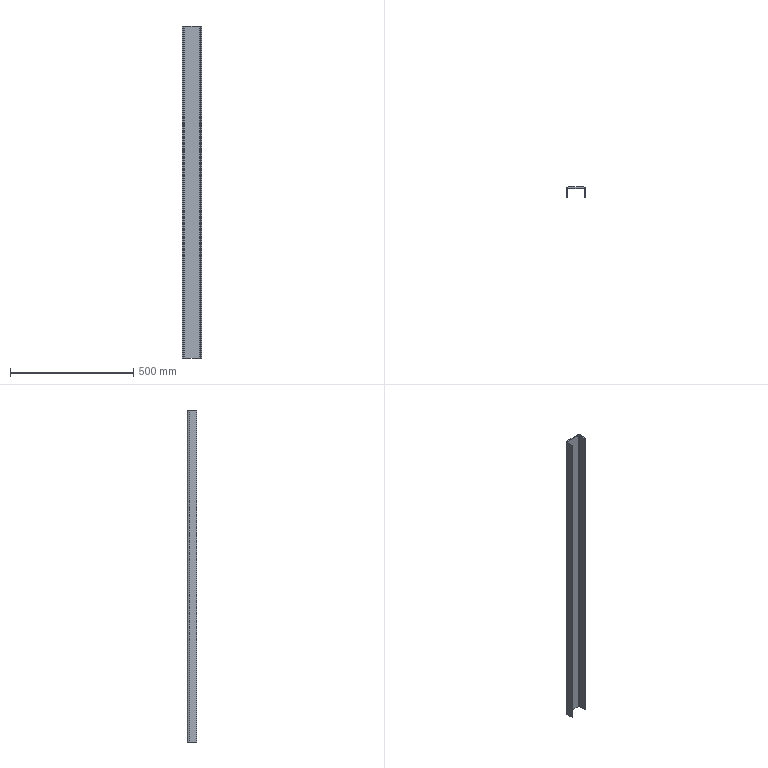Part | STEP file | 1 solid | 14 faces | box 80 x 40 x 1349 mm | volume 968325 mm3 | plane 10 | cylinder 4 | commonest cylinder face diameters 10 x2 20 x2
STEP:
#1=CARTESIAN_POINT('',(0.,0.,0.));
#2=DIRECTION('',(0.,0.,1.));
#3=DIRECTION('',(1.,0.,0.));
#4=AXIS2_PLACEMENT_3D('',#1,#2,#3);
#5=CARTESIAN_POINT('',(-35.,0.,674.5));
#6=VERTEX_POINT('',#5);
#7=CARTESIAN_POINT('',(-40.,0.,674.5));
#8=VERTEX_POINT('',#7);
#9=CARTESIAN_POINT('',(-30.,0.,674.5));
#10=DIRECTION('',(-1.,0.,0.));
#11=VECTOR('',#10,1.);
#12=LINE('',#9,#11);
#13=CARTESIAN_POINT('',(-35.,0.,674.5));
#14=DIRECTION('',(0.,-1.,0.));
#15=DIRECTION('',(0.,0.,-1.));
#16=AXIS2_PLACEMENT_3D('',#13,#14,#15);
#17=PLANE('',#16);
#18=CARTESIAN_POINT('',(0.,5.));
#19=DIRECTION('',(0.,-1.));
#20=VECTOR('',#19,1.);
#21=LINE('',#18,#20);
#22=(GEOMETRIC_REPRESENTATION_CONTEXT(2)PARAMETRIC_REPRESENTATION_CONTEXT()REPRESENTATION_CONTEXT('',''));
#23=DEFINITIONAL_REPRESENTATION('',(#21),#22);
#24=PCURVE('',#17,#23);
#25=CARTESIAN_POINT('',(-30.,30.,674.5));
#26=DIRECTION('',(0.,0.,-1.));
#27=DIRECTION('',(0.,-1.,0.));
#28=AXIS2_PLACEMENT_3D('',#25,#26,#27);
#29=PLANE('',#28);
#30=CARTESIAN_POINT('',(30.,0.));
#31=DIRECTION('',(0.,1.));
#32=VECTOR('',#31,1.);
#33=LINE('',#30,#32);
#34=(GEOMETRIC_REPRESENTATION_CONTEXT(2)PARAMETRIC_REPRESENTATION_CONTEXT()REPRESENTATION_CONTEXT('',''));
#35=DEFINITIONAL_REPRESENTATION('',(#33),#34);
#36=PCURVE('',#29,#35);
#37=SURFACE_CURVE('',#12,(#24,#36),.PCURVE_S1.);
#38=EDGE_CURVE('',#6,#8,#37,.T.);
#39=ORIENTED_EDGE('',*,*,#38,.T.);
#40=CARTESIAN_POINT('',(-40.,0.,-674.5));
#41=VERTEX_POINT('',#40);
#42=CARTESIAN_POINT('',(-40.,0.,674.5));
#43=DIRECTION('',(0.,0.,1.));
#44=VECTOR('',#43,1.);
#45=LINE('',#42,#44);
#46=CARTESIAN_POINT('',(0.,-5.));
#47=DIRECTION('',(-1.,0.));
#48=VECTOR('',#47,1.);
#49=LINE('',#46,#48);
#50=(GEOMETRIC_REPRESENTATION_CONTEXT(2)PARAMETRIC_REPRESENTATION_CONTEXT()REPRESENTATION_CONTEXT('',''));
#51=DEFINITIONAL_REPRESENTATION('',(#49),#50);
#52=PCURVE('',#17,#51);
#53=CARTESIAN_POINT('',(-40.,0.,674.5));
#54=DIRECTION('',(-1.,0.,0.));
#55=DIRECTION('',(0.,0.,1.));
#56=AXIS2_PLACEMENT_3D('',#53,#54,#55);
#57=PLANE('',#56);
#58=CARTESIAN_POINT('',(0.,0.));
#59=DIRECTION('',(1.,0.));
#60=VECTOR('',#59,1.);
#61=LINE('',#58,#60);
#62=(GEOMETRIC_REPRESENTATION_CONTEXT(2)PARAMETRIC_REPRESENTATION_CONTEXT()REPRESENTATION_CONTEXT('',''));
#63=DEFINITIONAL_REPRESENTATION('',(#61),#62);
#64=PCURVE('',#57,#63);
#65=SURFACE_CURVE('',#45,(#52,#64),.PCURVE_S1.);
#66=EDGE_CURVE('',#41,#8,#65,.T.);
#67=ORIENTED_EDGE('',*,*,#66,.F.);
#68=CARTESIAN_POINT('',(-35.,0.,-674.5));
#69=VERTEX_POINT('',#68);
#70=CARTESIAN_POINT('',(-30.,0.,-674.5));
#71=DIRECTION('',(-1.,0.,0.));
#72=VECTOR('',#71,1.);
#73=LINE('',#70,#72);
#74=CARTESIAN_POINT('',(1349.,5.));
#75=DIRECTION('',(0.,-1.));
#76=VECTOR('',#75,1.);
#77=LINE('',#74,#76);
#78=(GEOMETRIC_REPRESENTATION_CONTEXT(2)PARAMETRIC_REPRESENTATION_CONTEXT()REPRESENTATION_CONTEXT('',''));
#79=DEFINITIONAL_REPRESENTATION('',(#77),#78);
#80=PCURVE('',#17,#79);
#81=CARTESIAN_POINT('',(-30.,30.,-674.5));
#82=DIRECTION('',(0.,0.,-1.));
#83=DIRECTION('',(0.,-1.,0.));
#84=AXIS2_PLACEMENT_3D('',#81,#82,#83);
#85=PLANE('',#84);
#86=CARTESIAN_POINT('',(30.,0.));
#87=DIRECTION('',(0.,1.));
#88=VECTOR('',#87,1.);
#89=LINE('',#86,#88);
#90=(GEOMETRIC_REPRESENTATION_CONTEXT(2)PARAMETRIC_REPRESENTATION_CONTEXT()REPRESENTATION_CONTEXT('',''));
#91=DEFINITIONAL_REPRESENTATION('',(#89),#90);
#92=PCURVE('',#85,#91);
#93=SURFACE_CURVE('',#73,(#80,#92),.PCURVE_S1.);
#94=EDGE_CURVE('',#69,#41,#93,.T.);
#95=ORIENTED_EDGE('',*,*,#94,.F.);
#96=CARTESIAN_POINT('',(-35.,0.,674.5));
#97=DIRECTION('',(0.,0.,-1.));
#98=VECTOR('',#97,1.);
#99=LINE('',#96,#98);
#100=CARTESIAN_POINT('',(0.,0.));
#101=DIRECTION('',(1.,0.));
#102=VECTOR('',#101,1.);
#103=LINE('',#100,#102);
#104=(GEOMETRIC_REPRESENTATION_CONTEXT(2)PARAMETRIC_REPRESENTATION_CONTEXT()REPRESENTATION_CONTEXT('',''));
#105=DEFINITIONAL_REPRESENTATION('',(#103),#104);
#106=PCURVE('',#17,#105);
#107=CARTESIAN_POINT('',(-35.,30.,674.5));
#108=DIRECTION('',(1.,0.,0.));
#109=DIRECTION('',(0.,1.,0.));
#110=AXIS2_PLACEMENT_3D('',#107,#108,#109);
#111=PLANE('',#110);
#112=CARTESIAN_POINT('',(-30.,0.));
#113=DIRECTION('',(0.,-1.));
#114=VECTOR('',#113,1.);
#115=LINE('',#112,#114);
#116=(GEOMETRIC_REPRESENTATION_CONTEXT(2)PARAMETRIC_REPRESENTATION_CONTEXT()REPRESENTATION_CONTEXT('',''));
#117=DEFINITIONAL_REPRESENTATION('',(#115),#116);
#118=PCURVE('',#111,#117);
#119=SURFACE_CURVE('',#99,(#106,#118),.PCURVE_S1.);
#120=EDGE_CURVE('',#6,#69,#119,.T.);
#121=ORIENTED_EDGE('',*,*,#120,.F.);
#122=EDGE_LOOP('',(#39,#67,#95,#121));
#123=FACE_BOUND('',#122,.T.);
#124=ADVANCED_FACE('',(#123),#17,.T.);
#125=CARTESIAN_POINT('',(-40.,30.,674.5));
#126=VERTEX_POINT('',#125);
#127=CARTESIAN_POINT('',(-40.,30.,674.5));
#128=DIRECTION('',(0.,1.,0.));
#129=VECTOR('',#128,1.);
#130=LINE('',#127,#129);
#131=CARTESIAN_POINT('',(0.,30.));
#132=DIRECTION('',(0.,1.));
#133=VECTOR('',#132,1.);
#134=LINE('',#131,#133);
#135=(GEOMETRIC_REPRESENTATION_CONTEXT(2)PARAMETRIC_REPRESENTATION_CONTEXT()REPRESENTATION_CONTEXT('',''));
#136=DEFINITIONAL_REPRESENTATION('',(#134),#135);
#137=PCURVE('',#57,#136);
#138=CARTESIAN_POINT('',(0.,10.));
#139=DIRECTION('',(-1.,0.));
#140=VECTOR('',#139,1.);
#141=LINE('',#138,#140);
#142=(GEOMETRIC_REPRESENTATION_CONTEXT(2)PARAMETRIC_REPRESENTATION_CONTEXT()REPRESENTATION_CONTEXT('',''));
#143=DEFINITIONAL_REPRESENTATION('',(#141),#142);
#144=PCURVE('',#29,#143);
#145=SURFACE_CURVE('',#130,(#137,#144),.PCURVE_S1.);
#146=EDGE_CURVE('',#8,#126,#145,.T.);
#147=ORIENTED_EDGE('',*,*,#146,.T.);
#148=CARTESIAN_POINT('',(-40.,30.,-674.5));
#149=VERTEX_POINT('',#148);
#150=CARTESIAN_POINT('',(-40.,30.,674.5));
#151=DIRECTION('',(0.,0.,1.));
#152=VECTOR('',#151,1.);
#153=LINE('',#150,#152);
#154=CARTESIAN_POINT('',(0.,30.));
#155=DIRECTION('',(1.,0.));
#156=VECTOR('',#155,1.);
#157=LINE('',#154,#156);
#158=(GEOMETRIC_REPRESENTATION_CONTEXT(2)PARAMETRIC_REPRESENTATION_CONTEXT()REPRESENTATION_CONTEXT('',''));
#159=DEFINITIONAL_REPRESENTATION('',(#157),#158);
#160=PCURVE('',#57,#159);
#161=CARTESIAN_POINT('',(-30.,30.,674.5));
#162=DIRECTION('',(0.,0.,-1.));
#163=DIRECTION('',(-1.,0.,0.));
#164=AXIS2_PLACEMENT_3D('',#161,#162,#163);
#165=CYLINDRICAL_SURFACE('',#164,10.);
#166=CARTESIAN_POINT('',(0.,0.));
#167=DIRECTION('',(0.,-1.));
#168=VECTOR('',#167,1.);
#169=LINE('',#166,#168);
#170=(GEOMETRIC_REPRESENTATION_CONTEXT(2)PARAMETRIC_REPRESENTATION_CONTEXT()REPRESENTATION_CONTEXT('',''));
#171=DEFINITIONAL_REPRESENTATION('',(#169),#170);
#172=PCURVE('',#165,#171);
#173=SURFACE_CURVE('',#153,(#160,#172),.PCURVE_S1.);
#174=EDGE_CURVE('',#149,#126,#173,.T.);
#175=ORIENTED_EDGE('',*,*,#174,.F.);
#176=CARTESIAN_POINT('',(-40.,30.,-674.5));
#177=DIRECTION('',(0.,1.,0.));
#178=VECTOR('',#177,1.);
#179=LINE('',#176,#178);
#180=CARTESIAN_POINT('',(-1349.,30.));
#181=DIRECTION('',(0.,1.));
#182=VECTOR('',#181,1.);
#183=LINE('',#180,#182);
#184=(GEOMETRIC_REPRESENTATION_CONTEXT(2)PARAMETRIC_REPRESENTATION_CONTEXT()REPRESENTATION_CONTEXT('',''));
#185=DEFINITIONAL_REPRESENTATION('',(#183),#184);
#186=PCURVE('',#57,#185);
#187=CARTESIAN_POINT('',(0.,10.));
#188=DIRECTION('',(-1.,0.));
#189=VECTOR('',#188,1.);
#190=LINE('',#187,#189);
#191=(GEOMETRIC_REPRESENTATION_CONTEXT(2)PARAMETRIC_REPRESENTATION_CONTEXT()REPRESENTATION_CONTEXT('',''));
#192=DEFINITIONAL_REPRESENTATION('',(#190),#191);
#193=PCURVE('',#85,#192);
#194=SURFACE_CURVE('',#179,(#186,#193),.PCURVE_S1.);
#195=EDGE_CURVE('',#41,#149,#194,.T.);
#196=ORIENTED_EDGE('',*,*,#195,.F.);
#197=ORIENTED_EDGE('',*,*,#66,.T.);
#198=EDGE_LOOP('',(#147,#175,#196,#197));
#199=FACE_BOUND('',#198,.T.);
#200=ADVANCED_FACE('',(#199),#57,.T.);
#201=CARTESIAN_POINT('',(-30.,40.,674.5));
#202=VERTEX_POINT('',#201);
#203=CARTESIAN_POINT('',(-30.,30.,674.5));
#204=DIRECTION('',(0.,0.,-1.));
#205=DIRECTION('',(-1.,0.,0.));
#206=AXIS2_PLACEMENT_3D('',#203,#204,#205);
#207=CIRCLE('',#206,10.);
#208=CARTESIAN_POINT('',(0.,0.));
#209=DIRECTION('',(1.,0.));
#210=VECTOR('',#209,1.);
#211=LINE('',#208,#210);
#212=(GEOMETRIC_REPRESENTATION_CONTEXT(2)PARAMETRIC_REPRESENTATION_CONTEXT()REPRESENTATION_CONTEXT('',''));
#213=DEFINITIONAL_REPRESENTATION('',(#211),#212);
#214=PCURVE('',#165,#213);
#215=CARTESIAN_POINT('',(0.,0.));
#216=DIRECTION('',(0.,1.));
#217=AXIS2_PLACEMENT_2D('',#215,#216);
#218=CIRCLE('',#217,10.);
#219=(GEOMETRIC_REPRESENTATION_CONTEXT(2)PARAMETRIC_REPRESENTATION_CONTEXT()REPRESENTATION_CONTEXT('',''));
#220=DEFINITIONAL_REPRESENTATION('',(#218),#219);
#221=PCURVE('',#29,#220);
#222=SURFACE_CURVE('',#207,(#214,#221),.PCURVE_S1.);
#223=EDGE_CURVE('',#126,#202,#222,.T.);
#224=ORIENTED_EDGE('',*,*,#223,.T.);
#225=CARTESIAN_POINT('',(-30.,40.,-674.5));
#226=VERTEX_POINT('',#225);
#227=CARTESIAN_POINT('',(-30.,40.,674.5));
#228=DIRECTION('',(0.,0.,1.));
#229=VECTOR('',#228,1.);
#230=LINE('',#227,#229);
#231=CARTESIAN_POINT('',(1.571,0.));
#232=DIRECTION('',(0.,-1.));
#233=VECTOR('',#232,1.);
#234=LINE('',#231,#233);
#235=(GEOMETRIC_REPRESENTATION_CONTEXT(2)PARAMETRIC_REPRESENTATION_CONTEXT()REPRESENTATION_CONTEXT('',''));
#236=DEFINITIONAL_REPRESENTATION('',(#234),#235);
#237=PCURVE('',#165,#236);
#238=CARTESIAN_POINT('',(-30.,40.,674.5));
#239=DIRECTION('',(0.,1.,0.));
#240=DIRECTION('',(1.,0.,0.));
#241=AXIS2_PLACEMENT_3D('',#238,#239,#240);
#242=PLANE('',#241);
#243=CARTESIAN_POINT('',(0.,0.));
#244=DIRECTION('',(0.,-1.));
#245=VECTOR('',#244,1.);
#246=LINE('',#243,#245);
#247=(GEOMETRIC_REPRESENTATION_CONTEXT(2)PARAMETRIC_REPRESENTATION_CONTEXT()REPRESENTATION_CONTEXT('',''));
#248=DEFINITIONAL_REPRESENTATION('',(#246),#247);
#249=PCURVE('',#242,#248);
#250=SURFACE_CURVE('',#230,(#237,#249),.PCURVE_S1.);
#251=EDGE_CURVE('',#226,#202,#250,.T.);
#252=ORIENTED_EDGE('',*,*,#251,.F.);
#253=CARTESIAN_POINT('',(-30.,30.,-674.5));
#254=DIRECTION('',(0.,0.,-1.));
#255=DIRECTION('',(-1.,0.,0.));
#256=AXIS2_PLACEMENT_3D('',#253,#254,#255);
#257=CIRCLE('',#256,10.);
#258=CARTESIAN_POINT('',(0.,1349.));
#259=DIRECTION('',(1.,0.));
#260=VECTOR('',#259,1.);
#261=LINE('',#258,#260);
#262=(GEOMETRIC_REPRESENTATION_CONTEXT(2)PARAMETRIC_REPRESENTATION_CONTEXT()REPRESENTATION_CONTEXT('',''));
#263=DEFINITIONAL_REPRESENTATION('',(#261),#262);
#264=PCURVE('',#165,#263);
#265=CARTESIAN_POINT('',(0.,0.));
#266=DIRECTION('',(0.,1.));
#267=AXIS2_PLACEMENT_2D('',#265,#266);
#268=CIRCLE('',#267,10.);
#269=(GEOMETRIC_REPRESENTATION_CONTEXT(2)PARAMETRIC_REPRESENTATION_CONTEXT()REPRESENTATION_CONTEXT('',''));
#270=DEFINITIONAL_REPRESENTATION('',(#268),#269);
#271=PCURVE('',#85,#270);
#272=SURFACE_CURVE('',#257,(#264,#271),.PCURVE_S1.);
#273=EDGE_CURVE('',#149,#226,#272,.T.);
#274=ORIENTED_EDGE('',*,*,#273,.F.);
#275=ORIENTED_EDGE('',*,*,#174,.T.);
#276=EDGE_LOOP('',(#224,#252,#274,#275));
#277=FACE_BOUND('',#276,.T.);
#278=ADVANCED_FACE('',(#277),#165,.T.);
#279=CARTESIAN_POINT('',(30.,40.,674.5));
#280=VERTEX_POINT('',#279);
#281=CARTESIAN_POINT('',(-30.,40.,674.5));
#282=DIRECTION('',(1.,0.,0.));
#283=VECTOR('',#282,1.);
#284=LINE('',#281,#283);
#285=CARTESIAN_POINT('',(0.,0.));
#286=DIRECTION('',(1.,0.));
#287=VECTOR('',#286,1.);
#288=LINE('',#285,#287);
#289=(GEOMETRIC_REPRESENTATION_CONTEXT(2)PARAMETRIC_REPRESENTATION_CONTEXT()REPRESENTATION_CONTEXT('',''));
#290=DEFINITIONAL_REPRESENTATION('',(#288),#289);
#291=PCURVE('',#242,#290);
#292=CARTESIAN_POINT('',(-10.,0.));
#293=DIRECTION('',(0.,-1.));
#294=VECTOR('',#293,1.);
#295=LINE('',#292,#294);
#296=(GEOMETRIC_REPRESENTATION_CONTEXT(2)PARAMETRIC_REPRESENTATION_CONTEXT()REPRESENTATION_CONTEXT('',''));
#297=DEFINITIONAL_REPRESENTATION('',(#295),#296);
#298=PCURVE('',#29,#297);
#299=SURFACE_CURVE('',#284,(#291,#298),.PCURVE_S1.);
#300=EDGE_CURVE('',#202,#280,#299,.T.);
#301=ORIENTED_EDGE('',*,*,#300,.T.);
#302=CARTESIAN_POINT('',(30.,40.,-674.5));
#303=VERTEX_POINT('',#302);
#304=CARTESIAN_POINT('',(30.,40.,674.5));
#305=DIRECTION('',(0.,0.,1.));
#306=VECTOR('',#305,1.);
#307=LINE('',#304,#306);
#308=CARTESIAN_POINT('',(60.,0.));
#309=DIRECTION('',(0.,-1.));
#310=VECTOR('',#309,1.);
#311=LINE('',#308,#310);
#312=(GEOMETRIC_REPRESENTATION_CONTEXT(2)PARAMETRIC_REPRESENTATION_CONTEXT()REPRESENTATION_CONTEXT('',''));
#313=DEFINITIONAL_REPRESENTATION('',(#311),#312);
#314=PCURVE('',#242,#313);
#315=CARTESIAN_POINT('',(30.,30.,674.5));
#316=DIRECTION('',(0.,0.,-1.));
#317=DIRECTION('',(-1.,0.,0.));
#318=AXIS2_PLACEMENT_3D('',#315,#316,#317);
#319=CYLINDRICAL_SURFACE('',#318,10.);
#320=CARTESIAN_POINT('',(1.571,0.));
#321=DIRECTION('',(0.,-1.));
#322=VECTOR('',#321,1.);
#323=LINE('',#320,#322);
#324=(GEOMETRIC_REPRESENTATION_CONTEXT(2)PARAMETRIC_REPRESENTATION_CONTEXT()REPRESENTATION_CONTEXT('',''));
#325=DEFINITIONAL_REPRESENTATION('',(#323),#324);
#326=PCURVE('',#319,#325);
#327=SURFACE_CURVE('',#307,(#314,#326),.PCURVE_S1.);
#328=EDGE_CURVE('',#303,#280,#327,.T.);
#329=ORIENTED_EDGE('',*,*,#328,.F.);
#330=CARTESIAN_POINT('',(-30.,40.,-674.5));
#331=DIRECTION('',(1.,0.,0.));
#332=VECTOR('',#331,1.);
#333=LINE('',#330,#332);
#334=CARTESIAN_POINT('',(0.,1349.));
#335=DIRECTION('',(1.,0.));
#336=VECTOR('',#335,1.);
#337=LINE('',#334,#336);
#338=(GEOMETRIC_REPRESENTATION_CONTEXT(2)PARAMETRIC_REPRESENTATION_CONTEXT()REPRESENTATION_CONTEXT('',''));
#339=DEFINITIONAL_REPRESENTATION('',(#337),#338);
#340=PCURVE('',#242,#339);
#341=CARTESIAN_POINT('',(-10.,0.));
#342=DIRECTION('',(0.,-1.));
#343=VECTOR('',#342,1.);
#344=LINE('',#341,#343);
#345=(GEOMETRIC_REPRESENTATION_CONTEXT(2)PARAMETRIC_REPRESENTATION_CONTEXT()REPRESENTATION_CONTEXT('',''));
#346=DEFINITIONAL_REPRESENTATION('',(#344),#345);
#347=PCURVE('',#85,#346);
#348=SURFACE_CURVE('',#333,(#340,#347),.PCURVE_S1.);
#349=EDGE_CURVE('',#226,#303,#348,.T.);
#350=ORIENTED_EDGE('',*,*,#349,.F.);
#351=ORIENTED_EDGE('',*,*,#251,.T.);
#352=EDGE_LOOP('',(#301,#329,#350,#351));
#353=FACE_BOUND('',#352,.T.);
#354=ADVANCED_FACE('',(#353),#242,.T.);
#355=CARTESIAN_POINT('',(40.,30.,674.5));
#356=VERTEX_POINT('',#355);
#357=CARTESIAN_POINT('',(30.,30.,674.5));
#358=DIRECTION('',(0.,0.,-1.));
#359=DIRECTION('',(-1.,0.,0.));
#360=AXIS2_PLACEMENT_3D('',#357,#358,#359);
#361=CIRCLE('',#360,10.);
#362=CARTESIAN_POINT('',(0.,0.));
#363=DIRECTION('',(1.,0.));
#364=VECTOR('',#363,1.);
#365=LINE('',#362,#364);
#366=(GEOMETRIC_REPRESENTATION_CONTEXT(2)PARAMETRIC_REPRESENTATION_CONTEXT()REPRESENTATION_CONTEXT('',''));
#367=DEFINITIONAL_REPRESENTATION('',(#365),#366);
#368=PCURVE('',#319,#367);
#369=CARTESIAN_POINT('',(0.,-60.));
#370=DIRECTION('',(0.,1.));
#371=AXIS2_PLACEMENT_2D('',#369,#370);
#372=CIRCLE('',#371,10.);
#373=(GEOMETRIC_REPRESENTATION_CONTEXT(2)PARAMETRIC_REPRESENTATION_CONTEXT()REPRESENTATION_CONTEXT('',''));
#374=DEFINITIONAL_REPRESENTATION('',(#372),#373);
#375=PCURVE('',#29,#374);
#376=SURFACE_CURVE('',#361,(#368,#375),.PCURVE_S1.);
#377=EDGE_CURVE('',#280,#356,#376,.T.);
#378=ORIENTED_EDGE('',*,*,#377,.T.);
#379=CARTESIAN_POINT('',(40.,30.,-674.5));
#380=VERTEX_POINT('',#379);
#381=CARTESIAN_POINT('',(40.,30.,674.5));
#382=DIRECTION('',(0.,0.,1.));
#383=VECTOR('',#382,1.);
#384=LINE('',#381,#383);
#385=CARTESIAN_POINT('',(3.142,0.));
#386=DIRECTION('',(0.,-1.));
#387=VECTOR('',#386,1.);
#388=LINE('',#385,#387);
#389=(GEOMETRIC_REPRESENTATION_CONTEXT(2)PARAMETRIC_REPRESENTATION_CONTEXT()REPRESENTATION_CONTEXT('',''));
#390=DEFINITIONAL_REPRESENTATION('',(#388),#389);
#391=PCURVE('',#319,#390);
#392=CARTESIAN_POINT('',(40.,30.,674.5));
#393=DIRECTION('',(1.,0.,0.));
#394=DIRECTION('',(0.,-1.,0.));
#395=AXIS2_PLACEMENT_3D('',#392,#393,#394);
#396=PLANE('',#395);
#397=CARTESIAN_POINT('',(0.,0.));
#398=DIRECTION('',(0.,-1.));
#399=VECTOR('',#398,1.);
#400=LINE('',#397,#399);
#401=(GEOMETRIC_REPRESENTATION_CONTEXT(2)PARAMETRIC_REPRESENTATION_CONTEXT()REPRESENTATION_CONTEXT('',''));
#402=DEFINITIONAL_REPRESENTATION('',(#400),#401);
#403=PCURVE('',#396,#402);
#404=SURFACE_CURVE('',#384,(#391,#403),.PCURVE_S1.);
#405=EDGE_CURVE('',#380,#356,#404,.T.);
#406=ORIENTED_EDGE('',*,*,#405,.F.);
#407=CARTESIAN_POINT('',(30.,30.,-674.5));
#408=DIRECTION('',(0.,0.,-1.));
#409=DIRECTION('',(-1.,0.,0.));
#410=AXIS2_PLACEMENT_3D('',#407,#408,#409);
#411=CIRCLE('',#410,10.);
#412=CARTESIAN_POINT('',(0.,1349.));
#413=DIRECTION('',(1.,0.));
#414=VECTOR('',#413,1.);
#415=LINE('',#412,#414);
#416=(GEOMETRIC_REPRESENTATION_CONTEXT(2)PARAMETRIC_REPRESENTATION_CONTEXT()REPRESENTATION_CONTEXT('',''));
#417=DEFINITIONAL_REPRESENTATION('',(#415),#416);
#418=PCURVE('',#319,#417);
#419=CARTESIAN_POINT('',(0.,-60.));
#420=DIRECTION('',(0.,1.));
#421=AXIS2_PLACEMENT_2D('',#419,#420);
#422=CIRCLE('',#421,10.);
#423=(GEOMETRIC_REPRESENTATION_CONTEXT(2)PARAMETRIC_REPRESENTATION_CONTEXT()REPRESENTATION_CONTEXT('',''));
#424=DEFINITIONAL_REPRESENTATION('',(#422),#423);
#425=PCURVE('',#85,#424);
#426=SURFACE_CURVE('',#411,(#418,#425),.PCURVE_S1.);
#427=EDGE_CURVE('',#303,#380,#426,.T.);
#428=ORIENTED_EDGE('',*,*,#427,.F.);
#429=ORIENTED_EDGE('',*,*,#328,.T.);
#430=EDGE_LOOP('',(#378,#406,#428,#429));
#431=FACE_BOUND('',#430,.T.);
#432=ADVANCED_FACE('',(#431),#319,.T.);
#433=CARTESIAN_POINT('',(40.,0.,674.5));
#434=VERTEX_POINT('',#433);
#435=CARTESIAN_POINT('',(40.,30.,674.5));
#436=DIRECTION('',(0.,-1.,0.));
#437=VECTOR('',#436,1.);
#438=LINE('',#435,#437);
#439=CARTESIAN_POINT('',(0.,0.));
#440=DIRECTION('',(1.,0.));
#441=VECTOR('',#440,1.);
#442=LINE('',#439,#441);
#443=(GEOMETRIC_REPRESENTATION_CONTEXT(2)PARAMETRIC_REPRESENTATION_CONTEXT()REPRESENTATION_CONTEXT('',''));
#444=DEFINITIONAL_REPRESENTATION('',(#442),#443);
#445=PCURVE('',#396,#444);
#446=CARTESIAN_POINT('',(0.,-70.));
#447=DIRECTION('',(1.,0.));
#448=VECTOR('',#447,1.);
#449=LINE('',#446,#448);
#450=(GEOMETRIC_REPRESENTATION_CONTEXT(2)PARAMETRIC_REPRESENTATION_CONTEXT()REPRESENTATION_CONTEXT('',''));
#451=DEFINITIONAL_REPRESENTATION('',(#449),#450);
#452=PCURVE('',#29,#451);
#453=SURFACE_CURVE('',#438,(#445,#452),.PCURVE_S1.);
#454=EDGE_CURVE('',#356,#434,#453,.T.);
#455=ORIENTED_EDGE('',*,*,#454,.T.);
#456=CARTESIAN_POINT('',(40.,0.,-674.5));
#457=VERTEX_POINT('',#456);
#458=CARTESIAN_POINT('',(40.,0.,674.5));
#459=DIRECTION('',(0.,0.,1.));
#460=VECTOR('',#459,1.);
#461=LINE('',#458,#460);
#462=CARTESIAN_POINT('',(30.,0.));
#463=DIRECTION('',(0.,-1.));
#464=VECTOR('',#463,1.);
#465=LINE('',#462,#464);
#466=(GEOMETRIC_REPRESENTATION_CONTEXT(2)PARAMETRIC_REPRESENTATION_CONTEXT()REPRESENTATION_CONTEXT('',''));
#467=DEFINITIONAL_REPRESENTATION('',(#465),#466);
#468=PCURVE('',#396,#467);
#469=CARTESIAN_POINT('',(40.,0.,674.5));
#470=DIRECTION('',(0.,-1.,0.));
#471=DIRECTION('',(0.,0.,-1.));
#472=AXIS2_PLACEMENT_3D('',#469,#470,#471);
#473=PLANE('',#472);
#474=CARTESIAN_POINT('',(0.,0.));
#475=DIRECTION('',(-1.,0.));
#476=VECTOR('',#475,1.);
#477=LINE('',#474,#476);
#478=(GEOMETRIC_REPRESENTATION_CONTEXT(2)PARAMETRIC_REPRESENTATION_CONTEXT()REPRESENTATION_CONTEXT('',''));
#479=DEFINITIONAL_REPRESENTATION('',(#477),#478);
#480=PCURVE('',#473,#479);
#481=SURFACE_CURVE('',#461,(#468,#480),.PCURVE_S1.);
#482=EDGE_CURVE('',#457,#434,#481,.T.);
#483=ORIENTED_EDGE('',*,*,#482,.F.);
#484=CARTESIAN_POINT('',(40.,30.,-674.5));
#485=DIRECTION('',(0.,-1.,0.));
#486=VECTOR('',#485,1.);
#487=LINE('',#484,#486);
#488=CARTESIAN_POINT('',(0.,1349.));
#489=DIRECTION('',(1.,0.));
#490=VECTOR('',#489,1.);
#491=LINE('',#488,#490);
#492=(GEOMETRIC_REPRESENTATION_CONTEXT(2)PARAMETRIC_REPRESENTATION_CONTEXT()REPRESENTATION_CONTEXT('',''));
#493=DEFINITIONAL_REPRESENTATION('',(#491),#492);
#494=PCURVE('',#396,#493);
#495=CARTESIAN_POINT('',(0.,-70.));
#496=DIRECTION('',(1.,0.));
#497=VECTOR('',#496,1.);
#498=LINE('',#495,#497);
#499=(GEOMETRIC_REPRESENTATION_CONTEXT(2)PARAMETRIC_REPRESENTATION_CONTEXT()REPRESENTATION_CONTEXT('',''));
#500=DEFINITIONAL_REPRESENTATION('',(#498),#499);
#501=PCURVE('',#85,#500);
#502=SURFACE_CURVE('',#487,(#494,#501),.PCURVE_S1.);
#503=EDGE_CURVE('',#380,#457,#502,.T.);
#504=ORIENTED_EDGE('',*,*,#503,.F.);
#505=ORIENTED_EDGE('',*,*,#405,.T.);
#506=EDGE_LOOP('',(#455,#483,#504,#505));
#507=FACE_BOUND('',#506,.T.);
#508=ADVANCED_FACE('',(#507),#396,.T.);
#509=CARTESIAN_POINT('',(35.,0.,674.5));
#510=VERTEX_POINT('',#509);
#511=CARTESIAN_POINT('',(-30.,0.,674.5));
#512=DIRECTION('',(-1.,0.,0.));
#513=VECTOR('',#512,1.);
#514=LINE('',#511,#513);
#515=CARTESIAN_POINT('',(0.,-70.));
#516=DIRECTION('',(0.,-1.));
#517=VECTOR('',#516,1.);
#518=LINE('',#515,#517);
#519=(GEOMETRIC_REPRESENTATION_CONTEXT(2)PARAMETRIC_REPRESENTATION_CONTEXT()REPRESENTATION_CONTEXT('',''));
#520=DEFINITIONAL_REPRESENTATION('',(#518),#519);
#521=PCURVE('',#473,#520);
#522=CARTESIAN_POINT('',(30.,0.));
#523=DIRECTION('',(0.,1.));
#524=VECTOR('',#523,1.);
#525=LINE('',#522,#524);
#526=(GEOMETRIC_REPRESENTATION_CONTEXT(2)PARAMETRIC_REPRESENTATION_CONTEXT()REPRESENTATION_CONTEXT('',''));
#527=DEFINITIONAL_REPRESENTATION('',(#525),#526);
#528=PCURVE('',#29,#527);
#529=SURFACE_CURVE('',#514,(#521,#528),.PCURVE_S1.);
#530=EDGE_CURVE('',#434,#510,#529,.T.);
#531=ORIENTED_EDGE('',*,*,#530,.T.);
#532=CARTESIAN_POINT('',(35.,0.,-674.5));
#533=VERTEX_POINT('',#532);
#534=CARTESIAN_POINT('',(35.,0.,674.5));
#535=DIRECTION('',(0.,0.,1.));
#536=VECTOR('',#535,1.);
#537=LINE('',#534,#536);
#538=CARTESIAN_POINT('',(0.,-5.));
#539=DIRECTION('',(-1.,0.));
#540=VECTOR('',#539,1.);
#541=LINE('',#538,#540);
#542=(GEOMETRIC_REPRESENTATION_CONTEXT(2)PARAMETRIC_REPRESENTATION_CONTEXT()REPRESENTATION_CONTEXT('',''));
#543=DEFINITIONAL_REPRESENTATION('',(#541),#542);
#544=PCURVE('',#473,#543);
#545=CARTESIAN_POINT('',(35.,0.,674.5));
#546=DIRECTION('',(-1.,0.,0.));
#547=DIRECTION('',(0.,0.,1.));
#548=AXIS2_PLACEMENT_3D('',#545,#546,#547);
#549=PLANE('',#548);
#550=CARTESIAN_POINT('',(0.,0.));
#551=DIRECTION('',(1.,0.));
#552=VECTOR('',#551,1.);
#553=LINE('',#550,#552);
#554=(GEOMETRIC_REPRESENTATION_CONTEXT(2)PARAMETRIC_REPRESENTATION_CONTEXT()REPRESENTATION_CONTEXT('',''));
#555=DEFINITIONAL_REPRESENTATION('',(#553),#554);
#556=PCURVE('',#549,#555);
#557=SURFACE_CURVE('',#537,(#544,#556),.PCURVE_S1.);
#558=EDGE_CURVE('',#533,#510,#557,.T.);
#559=ORIENTED_EDGE('',*,*,#558,.F.);
#560=CARTESIAN_POINT('',(-30.,0.,-674.5));
#561=DIRECTION('',(-1.,0.,0.));
#562=VECTOR('',#561,1.);
#563=LINE('',#560,#562);
#564=CARTESIAN_POINT('',(1349.,-70.));
#565=DIRECTION('',(0.,-1.));
#566=VECTOR('',#565,1.);
#567=LINE('',#564,#566);
#568=(GEOMETRIC_REPRESENTATION_CONTEXT(2)PARAMETRIC_REPRESENTATION_CONTEXT()REPRESENTATION_CONTEXT('',''));
#569=DEFINITIONAL_REPRESENTATION('',(#567),#568);
#570=PCURVE('',#473,#569);
#571=CARTESIAN_POINT('',(30.,0.));
#572=DIRECTION('',(0.,1.));
#573=VECTOR('',#572,1.);
#574=LINE('',#571,#573);
#575=(GEOMETRIC_REPRESENTATION_CONTEXT(2)PARAMETRIC_REPRESENTATION_CONTEXT()REPRESENTATION_CONTEXT('',''));
#576=DEFINITIONAL_REPRESENTATION('',(#574),#575);
#577=PCURVE('',#85,#576);
#578=SURFACE_CURVE('',#563,(#570,#577),.PCURVE_S1.);
#579=EDGE_CURVE('',#457,#533,#578,.T.);
#580=ORIENTED_EDGE('',*,*,#579,.F.);
#581=ORIENTED_EDGE('',*,*,#482,.T.);
#582=EDGE_LOOP('',(#531,#559,#580,#581));
#583=FACE_BOUND('',#582,.T.);
#584=ADVANCED_FACE('',(#583),#473,.T.);
#585=CARTESIAN_POINT('',(35.,30.,674.5));
#586=VERTEX_POINT('',#585);
#587=CARTESIAN_POINT('',(35.,30.,674.5));
#588=DIRECTION('',(0.,1.,0.));
#589=VECTOR('',#588,1.);
#590=LINE('',#587,#589);
#591=CARTESIAN_POINT('',(0.,30.));
#592=DIRECTION('',(0.,1.));
#593=VECTOR('',#592,1.);
#594=LINE('',#591,#593);
#595=(GEOMETRIC_REPRESENTATION_CONTEXT(2)PARAMETRIC_REPRESENTATION_CONTEXT()REPRESENTATION_CONTEXT('',''));
#596=DEFINITIONAL_REPRESENTATION('',(#594),#595);
#597=PCURVE('',#549,#596);
#598=CARTESIAN_POINT('',(0.,-65.));
#599=DIRECTION('',(-1.,0.));
#600=VECTOR('',#599,1.);
#601=LINE('',#598,#600);
#602=(GEOMETRIC_REPRESENTATION_CONTEXT(2)PARAMETRIC_REPRESENTATION_CONTEXT()REPRESENTATION_CONTEXT('',''));
#603=DEFINITIONAL_REPRESENTATION('',(#601),#602);
#604=PCURVE('',#29,#603);
#605=SURFACE_CURVE('',#590,(#597,#604),.PCURVE_S1.);
#606=EDGE_CURVE('',#510,#586,#605,.T.);
#607=ORIENTED_EDGE('',*,*,#606,.T.);
#608=CARTESIAN_POINT('',(35.,30.,-674.5));
#609=VERTEX_POINT('',#608);
#610=CARTESIAN_POINT('',(35.,30.,674.5));
#611=DIRECTION('',(0.,0.,-1.));
#612=VECTOR('',#611,1.);
#613=LINE('',#610,#612);
#614=CARTESIAN_POINT('',(0.,30.));
#615=DIRECTION('',(-1.,0.));
#616=VECTOR('',#615,1.);
#617=LINE('',#614,#616);
#618=(GEOMETRIC_REPRESENTATION_CONTEXT(2)PARAMETRIC_REPRESENTATION_CONTEXT()REPRESENTATION_CONTEXT('',''));
#619=DEFINITIONAL_REPRESENTATION('',(#617),#618);
#620=PCURVE('',#549,#619);
#621=CARTESIAN_POINT('',(30.,30.,674.5));
#622=DIRECTION('',(0.,0.,-1.));
#623=DIRECTION('',(-1.,0.,0.));
#624=AXIS2_PLACEMENT_3D('',#621,#622,#623);
#625=CYLINDRICAL_SURFACE('',#624,5.);
#626=CARTESIAN_POINT('',(3.142,0.));
#627=DIRECTION('',(0.,1.));
#628=VECTOR('',#627,1.);
#629=LINE('',#626,#628);
#630=(GEOMETRIC_REPRESENTATION_CONTEXT(2)PARAMETRIC_REPRESENTATION_CONTEXT()REPRESENTATION_CONTEXT('',''));
#631=DEFINITIONAL_REPRESENTATION('',(#629),#630);
#632=PCURVE('',#625,#631);
#633=SURFACE_CURVE('',#613,(#620,#632),.PCURVE_S1.);
#634=EDGE_CURVE('',#586,#609,#633,.T.);
#635=ORIENTED_EDGE('',*,*,#634,.T.);
#636=CARTESIAN_POINT('',(35.,30.,-674.5));
#637=DIRECTION('',(0.,1.,0.));
#638=VECTOR('',#637,1.);
#639=LINE('',#636,#638);
#640=CARTESIAN_POINT('',(-1349.,30.));
#641=DIRECTION('',(0.,1.));
#642=VECTOR('',#641,1.);
#643=LINE('',#640,#642);
#644=(GEOMETRIC_REPRESENTATION_CONTEXT(2)PARAMETRIC_REPRESENTATION_CONTEXT()REPRESENTATION_CONTEXT('',''));
#645=DEFINITIONAL_REPRESENTATION('',(#643),#644);
#646=PCURVE('',#549,#645);
#647=CARTESIAN_POINT('',(0.,-65.));
#648=DIRECTION('',(-1.,0.));
#649=VECTOR('',#648,1.);
#650=LINE('',#647,#649);
#651=(GEOMETRIC_REPRESENTATION_CONTEXT(2)PARAMETRIC_REPRESENTATION_CONTEXT()REPRESENTATION_CONTEXT('',''));
#652=DEFINITIONAL_REPRESENTATION('',(#650),#651);
#653=PCURVE('',#85,#652);
#654=SURFACE_CURVE('',#639,(#646,#653),.PCURVE_S1.);
#655=EDGE_CURVE('',#533,#609,#654,.T.);
#656=ORIENTED_EDGE('',*,*,#655,.F.);
#657=ORIENTED_EDGE('',*,*,#558,.T.);
#658=EDGE_LOOP('',(#607,#635,#656,#657));
#659=FACE_BOUND('',#658,.T.);
#660=ADVANCED_FACE('',(#659),#549,.T.);
#661=CARTESIAN_POINT('',(-35.,30.,674.5));
#662=VERTEX_POINT('',#661);
#663=CARTESIAN_POINT('',(-35.,30.,674.5));
#664=DIRECTION('',(0.,-1.,0.));
#665=VECTOR('',#664,1.);
#666=LINE('',#663,#665);
#667=CARTESIAN_POINT('',(0.,0.));
#668=DIRECTION('',(-1.,0.));
#669=VECTOR('',#668,1.);
#670=LINE('',#667,#669);
#671=(GEOMETRIC_REPRESENTATION_CONTEXT(2)PARAMETRIC_REPRESENTATION_CONTEXT()REPRESENTATION_CONTEXT('',''));
#672=DEFINITIONAL_REPRESENTATION('',(#670),#671);
#673=PCURVE('',#111,#672);
#674=CARTESIAN_POINT('',(0.,5.));
#675=DIRECTION('',(1.,0.));
#676=VECTOR('',#675,1.);
#677=LINE('',#674,#676);
#678=(GEOMETRIC_REPRESENTATION_CONTEXT(2)PARAMETRIC_REPRESENTATION_CONTEXT()REPRESENTATION_CONTEXT('',''));
#679=DEFINITIONAL_REPRESENTATION('',(#677),#678);
#680=PCURVE('',#29,#679);
#681=SURFACE_CURVE('',#666,(#673,#680),.PCURVE_S1.);
#682=EDGE_CURVE('',#662,#6,#681,.T.);
#683=ORIENTED_EDGE('',*,*,#682,.T.);
#684=ORIENTED_EDGE('',*,*,#120,.T.);
#685=CARTESIAN_POINT('',(-35.,30.,-674.5));
#686=VERTEX_POINT('',#685);
#687=CARTESIAN_POINT('',(-35.,30.,-674.5));
#688=DIRECTION('',(0.,-1.,0.));
#689=VECTOR('',#688,1.);
#690=LINE('',#687,#689);
#691=CARTESIAN_POINT('',(0.,-1349.));
#692=DIRECTION('',(-1.,0.));
#693=VECTOR('',#692,1.);
#694=LINE('',#691,#693);
#695=(GEOMETRIC_REPRESENTATION_CONTEXT(2)PARAMETRIC_REPRESENTATION_CONTEXT()REPRESENTATION_CONTEXT('',''));
#696=DEFINITIONAL_REPRESENTATION('',(#694),#695);
#697=PCURVE('',#111,#696);
#698=CARTESIAN_POINT('',(0.,5.));
#699=DIRECTION('',(1.,0.));
#700=VECTOR('',#699,1.);
#701=LINE('',#698,#700);
#702=(GEOMETRIC_REPRESENTATION_CONTEXT(2)PARAMETRIC_REPRESENTATION_CONTEXT()REPRESENTATION_CONTEXT('',''));
#703=DEFINITIONAL_REPRESENTATION('',(#701),#702);
#704=PCURVE('',#85,#703);
#705=SURFACE_CURVE('',#690,(#697,#704),.PCURVE_S1.);
#706=EDGE_CURVE('',#686,#69,#705,.T.);
#707=ORIENTED_EDGE('',*,*,#706,.F.);
#708=CARTESIAN_POINT('',(-35.,30.,674.5));
#709=DIRECTION('',(0.,0.,1.));
#710=VECTOR('',#709,1.);
#711=LINE('',#708,#710);
#712=CARTESIAN_POINT('',(0.,0.));
#713=DIRECTION('',(0.,1.));
#714=VECTOR('',#713,1.);
#715=LINE('',#712,#714);
#716=(GEOMETRIC_REPRESENTATION_CONTEXT(2)PARAMETRIC_REPRESENTATION_CONTEXT()REPRESENTATION_CONTEXT('',''));
#717=DEFINITIONAL_REPRESENTATION('',(#715),#716);
#718=PCURVE('',#111,#717);
#719=CARTESIAN_POINT('',(-30.,30.,674.5));
#720=DIRECTION('',(0.,0.,-1.));
#721=DIRECTION('',(-1.,0.,0.));
#722=AXIS2_PLACEMENT_3D('',#719,#720,#721);
#723=CYLINDRICAL_SURFACE('',#722,5.);
#724=CARTESIAN_POINT('',(0.,0.));
#725=DIRECTION('',(0.,-1.));
#726=VECTOR('',#725,1.);
#727=LINE('',#724,#726);
#728=(GEOMETRIC_REPRESENTATION_CONTEXT(2)PARAMETRIC_REPRESENTATION_CONTEXT()REPRESENTATION_CONTEXT('',''));
#729=DEFINITIONAL_REPRESENTATION('',(#727),#728);
#730=PCURVE('',#723,#729);
#731=SURFACE_CURVE('',#711,(#718,#730),.PCURVE_S1.);
#732=EDGE_CURVE('',#686,#662,#731,.T.);
#733=ORIENTED_EDGE('',*,*,#732,.T.);
#734=EDGE_LOOP('',(#683,#684,#707,#733));
#735=FACE_BOUND('',#734,.T.);
#736=ADVANCED_FACE('',(#735),#111,.T.);
#737=CARTESIAN_POINT('',(-30.,35.,-674.5));
#738=VERTEX_POINT('',#737);
#739=CARTESIAN_POINT('',(30.,35.,-674.5));
#740=VERTEX_POINT('',#739);
#741=CARTESIAN_POINT('',(30.,35.,-674.5));
#742=DIRECTION('',(1.,0.,0.));
#743=VECTOR('',#742,1.);
#744=LINE('',#741,#743);
#745=CARTESIAN_POINT('',(-5.,-60.));
#746=DIRECTION('',(0.,-1.));
#747=VECTOR('',#746,1.);
#748=LINE('',#745,#747);
#749=(GEOMETRIC_REPRESENTATION_CONTEXT(2)PARAMETRIC_REPRESENTATION_CONTEXT()REPRESENTATION_CONTEXT('',''));
#750=DEFINITIONAL_REPRESENTATION('',(#748),#749);
#751=PCURVE('',#85,#750);
#752=CARTESIAN_POINT('',(30.,35.,674.5));
#753=DIRECTION('',(0.,-1.,0.));
#754=DIRECTION('',(0.,0.,-1.));
#755=AXIS2_PLACEMENT_3D('',#752,#753,#754);
#756=PLANE('',#755);
#757=CARTESIAN_POINT('',(1349.,0.));
#758=DIRECTION('',(0.,1.));
#759=VECTOR('',#758,1.);
#760=LINE('',#757,#759);
#761=(GEOMETRIC_REPRESENTATION_CONTEXT(2)PARAMETRIC_REPRESENTATION_CONTEXT()REPRESENTATION_CONTEXT('',''));
#762=DEFINITIONAL_REPRESENTATION('',(#760),#761);
#763=PCURVE('',#756,#762);
#764=SURFACE_CURVE('',#744,(#751,#763),.PCURVE_S1.);
#765=EDGE_CURVE('',#738,#740,#764,.T.);
#766=ORIENTED_EDGE('',*,*,#765,.F.);
#767=CARTESIAN_POINT('',(-30.,30.,-674.5));
#768=DIRECTION('',(0.,0.,1.));
#769=DIRECTION('',(-1.,0.,0.));
#770=AXIS2_PLACEMENT_3D('',#767,#768,#769);
#771=CIRCLE('',#770,5.);
#772=CARTESIAN_POINT('',(0.,5.));
#773=CARTESIAN_POINT('',(8.66,5.));
#774=CARTESIAN_POINT('',(4.33,-2.5));
#775=CARTESIAN_POINT('',(0.,-10.));
#776=CARTESIAN_POINT('',(-4.33,-2.5));
#777=CARTESIAN_POINT('',(-8.66,5.));
#778=CARTESIAN_POINT('',(0.,5.));
#779=(BOUNDED_CURVE()B_SPLINE_CURVE(2,(#772,#773,#774,#775,#776,#777,#778),.UNSPECIFIED.,.T.,.F.)B_SPLINE_CURVE_WITH_KNOTS((1,2,2,2,2,1),(-2.094,0.,2.094,4.189,6.283,8.378),.UNSPECIFIED.)CURVE()GEOMETRIC_REPRESENTATION_ITEM()RATIONAL_B_SPLINE_CURVE((1.,0.5,1.,0.5,1.,0.5,1.))REPRESENTATION_ITEM(''));
#780=(GEOMETRIC_REPRESENTATION_CONTEXT(2)PARAMETRIC_REPRESENTATION_CONTEXT()REPRESENTATION_CONTEXT('',''));
#781=DEFINITIONAL_REPRESENTATION('',(#779),#780);
#782=PCURVE('',#85,#781);
#783=CARTESIAN_POINT('',(6.283,1349.));
#784=DIRECTION('',(-1.,0.));
#785=VECTOR('',#784,1.);
#786=LINE('',#783,#785);
#787=(GEOMETRIC_REPRESENTATION_CONTEXT(2)PARAMETRIC_REPRESENTATION_CONTEXT()REPRESENTATION_CONTEXT('',''));
#788=DEFINITIONAL_REPRESENTATION('',(#786),#787);
#789=PCURVE('',#723,#788);
#790=SURFACE_CURVE('',#771,(#782,#789),.PCURVE_S1.);
#791=EDGE_CURVE('',#738,#686,#790,.T.);
#792=ORIENTED_EDGE('',*,*,#791,.T.);
#793=ORIENTED_EDGE('',*,*,#706,.T.);
#794=ORIENTED_EDGE('',*,*,#94,.T.);
#795=ORIENTED_EDGE('',*,*,#195,.T.);
#796=ORIENTED_EDGE('',*,*,#273,.T.);
#797=ORIENTED_EDGE('',*,*,#349,.T.);
#798=ORIENTED_EDGE('',*,*,#427,.T.);
#799=ORIENTED_EDGE('',*,*,#503,.T.);
#800=ORIENTED_EDGE('',*,*,#579,.T.);
#801=ORIENTED_EDGE('',*,*,#655,.T.);
#802=CARTESIAN_POINT('',(30.,30.,-674.5));
#803=DIRECTION('',(0.,0.,1.));
#804=DIRECTION('',(-1.,0.,0.));
#805=AXIS2_PLACEMENT_3D('',#802,#803,#804);
#806=CIRCLE('',#805,5.);
#807=CARTESIAN_POINT('',(0.,-55.));
#808=CARTESIAN_POINT('',(8.66,-55.));
#809=CARTESIAN_POINT('',(4.33,-62.5));
#810=CARTESIAN_POINT('',(0.,-70.));
#811=CARTESIAN_POINT('',(-4.33,-62.5));
#812=CARTESIAN_POINT('',(-8.66,-55.));
#813=CARTESIAN_POINT('',(0.,-55.));
#814=(BOUNDED_CURVE()B_SPLINE_CURVE(2,(#807,#808,#809,#810,#811,#812,#813),.UNSPECIFIED.,.T.,.F.)B_SPLINE_CURVE_WITH_KNOTS((1,2,2,2,2,1),(-2.094,0.,2.094,4.189,6.283,8.378),.UNSPECIFIED.)CURVE()GEOMETRIC_REPRESENTATION_ITEM()RATIONAL_B_SPLINE_CURVE((1.,0.5,1.,0.5,1.,0.5,1.))REPRESENTATION_ITEM(''));
#815=(GEOMETRIC_REPRESENTATION_CONTEXT(2)PARAMETRIC_REPRESENTATION_CONTEXT()REPRESENTATION_CONTEXT('',''));
#816=DEFINITIONAL_REPRESENTATION('',(#814),#815);
#817=PCURVE('',#85,#816);
#818=CARTESIAN_POINT('',(6.283,1349.));
#819=DIRECTION('',(-1.,0.));
#820=VECTOR('',#819,1.);
#821=LINE('',#818,#820);
#822=(GEOMETRIC_REPRESENTATION_CONTEXT(2)PARAMETRIC_REPRESENTATION_CONTEXT()REPRESENTATION_CONTEXT('',''));
#823=DEFINITIONAL_REPRESENTATION('',(#821),#822);
#824=PCURVE('',#625,#823);
#825=SURFACE_CURVE('',#806,(#817,#824),.PCURVE_S1.);
#826=EDGE_CURVE('',#609,#740,#825,.T.);
#827=ORIENTED_EDGE('',*,*,#826,.T.);
#828=EDGE_LOOP('',(#766,#792,#793,#794,#795,#796,#797,#798,#799,#800,#801,#827));
#829=FACE_BOUND('',#828,.T.);
#830=ADVANCED_FACE('',(#829),#85,.T.);
#831=ORIENTED_EDGE('',*,*,#826,.T.);
#832=CARTESIAN_POINT('',(30.,35.,674.5));
#833=VERTEX_POINT('',#832);
#834=CARTESIAN_POINT('',(30.,35.,674.5));
#835=DIRECTION('',(0.,0.,1.));
#836=VECTOR('',#835,1.);
#837=LINE('',#834,#836);
#838=CARTESIAN_POINT('',(1.571,0.));
#839=DIRECTION('',(0.,-1.));
#840=VECTOR('',#839,1.);
#841=LINE('',#838,#840);
#842=(GEOMETRIC_REPRESENTATION_CONTEXT(2)PARAMETRIC_REPRESENTATION_CONTEXT()REPRESENTATION_CONTEXT('',''));
#843=DEFINITIONAL_REPRESENTATION('',(#841),#842);
#844=PCURVE('',#625,#843);
#845=CARTESIAN_POINT('',(0.,0.));
#846=DIRECTION('',(-1.,0.));
#847=VECTOR('',#846,1.);
#848=LINE('',#845,#847);
#849=(GEOMETRIC_REPRESENTATION_CONTEXT(2)PARAMETRIC_REPRESENTATION_CONTEXT()REPRESENTATION_CONTEXT('',''));
#850=DEFINITIONAL_REPRESENTATION('',(#848),#849);
#851=PCURVE('',#756,#850);
#852=SURFACE_CURVE('',#837,(#844,#851),.PCURVE_S1.);
#853=EDGE_CURVE('',#740,#833,#852,.T.);
#854=ORIENTED_EDGE('',*,*,#853,.T.);
#855=CARTESIAN_POINT('',(30.,30.,674.5));
#856=DIRECTION('',(0.,0.,1.));
#857=DIRECTION('',(-1.,0.,0.));
#858=AXIS2_PLACEMENT_3D('',#855,#856,#857);
#859=CIRCLE('',#858,5.);
#860=CARTESIAN_POINT('',(6.283,0.));
#861=DIRECTION('',(-1.,0.));
#862=VECTOR('',#861,1.);
#863=LINE('',#860,#862);
#864=(GEOMETRIC_REPRESENTATION_CONTEXT(2)PARAMETRIC_REPRESENTATION_CONTEXT()REPRESENTATION_CONTEXT('',''));
#865=DEFINITIONAL_REPRESENTATION('',(#863),#864);
#866=PCURVE('',#625,#865);
#867=CARTESIAN_POINT('',(0.,-55.));
#868=CARTESIAN_POINT('',(8.66,-55.));
#869=CARTESIAN_POINT('',(4.33,-62.5));
#870=CARTESIAN_POINT('',(0.,-70.));
#871=CARTESIAN_POINT('',(-4.33,-62.5));
#872=CARTESIAN_POINT('',(-8.66,-55.));
#873=CARTESIAN_POINT('',(0.,-55.));
#874=(BOUNDED_CURVE()B_SPLINE_CURVE(2,(#867,#868,#869,#870,#871,#872,#873),.UNSPECIFIED.,.T.,.F.)B_SPLINE_CURVE_WITH_KNOTS((1,2,2,2,2,1),(-2.094,0.,2.094,4.189,6.283,8.378),.UNSPECIFIED.)CURVE()GEOMETRIC_REPRESENTATION_ITEM()RATIONAL_B_SPLINE_CURVE((1.,0.5,1.,0.5,1.,0.5,1.))REPRESENTATION_ITEM(''));
#875=(GEOMETRIC_REPRESENTATION_CONTEXT(2)PARAMETRIC_REPRESENTATION_CONTEXT()REPRESENTATION_CONTEXT('',''));
#876=DEFINITIONAL_REPRESENTATION('',(#874),#875);
#877=PCURVE('',#29,#876);
#878=SURFACE_CURVE('',#859,(#866,#877),.PCURVE_S1.);
#879=EDGE_CURVE('',#586,#833,#878,.T.);
#880=ORIENTED_EDGE('',*,*,#879,.F.);
#881=ORIENTED_EDGE('',*,*,#634,.T.);
#882=EDGE_LOOP('',(#831,#854,#880,#881));
#883=FACE_BOUND('',#882,.F.);
#884=ADVANCED_FACE('',(#883),#625,.F.);
#885=CARTESIAN_POINT('',(-30.,35.,674.5));
#886=VERTEX_POINT('',#885);
#887=CARTESIAN_POINT('',(-30.,30.,674.5));
#888=DIRECTION('',(0.,0.,-1.));
#889=DIRECTION('',(-1.,0.,0.));
#890=AXIS2_PLACEMENT_3D('',#887,#888,#889);
#891=CIRCLE('',#890,5.);
#892=CARTESIAN_POINT('',(0.,0.));
#893=DIRECTION('',(0.,1.));
#894=AXIS2_PLACEMENT_2D('',#892,#893);
#895=CIRCLE('',#894,5.);
#896=(GEOMETRIC_REPRESENTATION_CONTEXT(2)PARAMETRIC_REPRESENTATION_CONTEXT()REPRESENTATION_CONTEXT('',''));
#897=DEFINITIONAL_REPRESENTATION('',(#895),#896);
#898=PCURVE('',#29,#897);
#899=CARTESIAN_POINT('',(0.,0.));
#900=DIRECTION('',(1.,0.));
#901=VECTOR('',#900,1.);
#902=LINE('',#899,#901);
#903=(GEOMETRIC_REPRESENTATION_CONTEXT(2)PARAMETRIC_REPRESENTATION_CONTEXT()REPRESENTATION_CONTEXT('',''));
#904=DEFINITIONAL_REPRESENTATION('',(#902),#903);
#905=PCURVE('',#723,#904);
#906=SURFACE_CURVE('',#891,(#898,#905),.PCURVE_S1.);
#907=EDGE_CURVE('',#662,#886,#906,.T.);
#908=ORIENTED_EDGE('',*,*,#907,.T.);
#909=CARTESIAN_POINT('',(30.,35.,674.5));
#910=DIRECTION('',(-1.,0.,0.));
#911=VECTOR('',#910,1.);
#912=LINE('',#909,#911);
#913=CARTESIAN_POINT('',(-5.,-60.));
#914=DIRECTION('',(0.,1.));
#915=VECTOR('',#914,1.);
#916=LINE('',#913,#915);
#917=(GEOMETRIC_REPRESENTATION_CONTEXT(2)PARAMETRIC_REPRESENTATION_CONTEXT()REPRESENTATION_CONTEXT('',''));
#918=DEFINITIONAL_REPRESENTATION('',(#916),#917);
#919=PCURVE('',#29,#918);
#920=CARTESIAN_POINT('',(0.,0.));
#921=DIRECTION('',(0.,-1.));
#922=VECTOR('',#921,1.);
#923=LINE('',#920,#922);
#924=(GEOMETRIC_REPRESENTATION_CONTEXT(2)PARAMETRIC_REPRESENTATION_CONTEXT()REPRESENTATION_CONTEXT('',''));
#925=DEFINITIONAL_REPRESENTATION('',(#923),#924);
#926=PCURVE('',#756,#925);
#927=SURFACE_CURVE('',#912,(#919,#926),.PCURVE_S1.);
#928=EDGE_CURVE('',#833,#886,#927,.T.);
#929=ORIENTED_EDGE('',*,*,#928,.F.);
#930=ORIENTED_EDGE('',*,*,#879,.F.);
#931=ORIENTED_EDGE('',*,*,#606,.F.);
#932=ORIENTED_EDGE('',*,*,#530,.F.);
#933=ORIENTED_EDGE('',*,*,#454,.F.);
#934=ORIENTED_EDGE('',*,*,#377,.F.);
#935=ORIENTED_EDGE('',*,*,#300,.F.);
#936=ORIENTED_EDGE('',*,*,#223,.F.);
#937=ORIENTED_EDGE('',*,*,#146,.F.);
#938=ORIENTED_EDGE('',*,*,#38,.F.);
#939=ORIENTED_EDGE('',*,*,#682,.F.);
#940=EDGE_LOOP('',(#908,#929,#930,#931,#932,#933,#934,#935,#936,#937,#938,#939));
#941=FACE_BOUND('',#940,.T.);
#942=ADVANCED_FACE('',(#941),#29,.F.);
#943=ORIENTED_EDGE('',*,*,#791,.T.);
#944=ORIENTED_EDGE('',*,*,#732,.T.);
#945=ORIENTED_EDGE('',*,*,#907,.T.);
#946=CARTESIAN_POINT('',(-30.,35.,674.5));
#947=DIRECTION('',(0.,0.,-1.));
#948=VECTOR('',#947,1.);
#949=LINE('',#946,#948);
#950=CARTESIAN_POINT('',(1.571,0.));
#951=DIRECTION('',(0.,1.));
#952=VECTOR('',#951,1.);
#953=LINE('',#950,#952);
#954=(GEOMETRIC_REPRESENTATION_CONTEXT(2)PARAMETRIC_REPRESENTATION_CONTEXT()REPRESENTATION_CONTEXT('',''));
#955=DEFINITIONAL_REPRESENTATION('',(#953),#954);
#956=PCURVE('',#723,#955);
#957=CARTESIAN_POINT('',(0.,-60.));
#958=DIRECTION('',(1.,0.));
#959=VECTOR('',#958,1.);
#960=LINE('',#957,#959);
#961=(GEOMETRIC_REPRESENTATION_CONTEXT(2)PARAMETRIC_REPRESENTATION_CONTEXT()REPRESENTATION_CONTEXT('',''));
#962=DEFINITIONAL_REPRESENTATION('',(#960),#961);
#963=PCURVE('',#756,#962);
#964=SURFACE_CURVE('',#949,(#956,#963),.PCURVE_S1.);
#965=EDGE_CURVE('',#886,#738,#964,.T.);
#966=ORIENTED_EDGE('',*,*,#965,.T.);
#967=EDGE_LOOP('',(#943,#944,#945,#966));
#968=FACE_BOUND('',#967,.F.);
#969=ADVANCED_FACE('',(#968),#723,.F.);
#970=ORIENTED_EDGE('',*,*,#928,.T.);
#971=ORIENTED_EDGE('',*,*,#965,.T.);
#972=ORIENTED_EDGE('',*,*,#765,.T.);
#973=ORIENTED_EDGE('',*,*,#853,.T.);
#974=EDGE_LOOP('',(#970,#971,#972,#973));
#975=FACE_BOUND('',#974,.T.);
#976=ADVANCED_FACE('',(#975),#756,.T.);
#977=CLOSED_SHELL('',(#124,#200,#278,#354,#432,#508,#584,#660,#736,#830,#884,#942,#969,#976));
#978=MANIFOLD_SOLID_BREP('',#977);
#979=(LENGTH_UNIT()NAMED_UNIT(*)SI_UNIT(.MILLI.,.METRE.));
#980=UNCERTAINTY_MEASURE_WITH_UNIT(LENGTH_MEASURE(0.0000001),#979,'','');
#981=(NAMED_UNIT(*)PLANE_ANGLE_UNIT()SI_UNIT($,.RADIAN.));
#982=(NAMED_UNIT(*)SI_UNIT($,.STERADIAN.)SOLID_ANGLE_UNIT());
#983=(GEOMETRIC_REPRESENTATION_CONTEXT(3)GLOBAL_UNCERTAINTY_ASSIGNED_CONTEXT((#980))GLOBAL_UNIT_ASSIGNED_CONTEXT((#979,#981,#982))REPRESENTATION_CONTEXT('',''));
#984=ADVANCED_BREP_SHAPE_REPRESENTATION('',(#4,#978),#983);